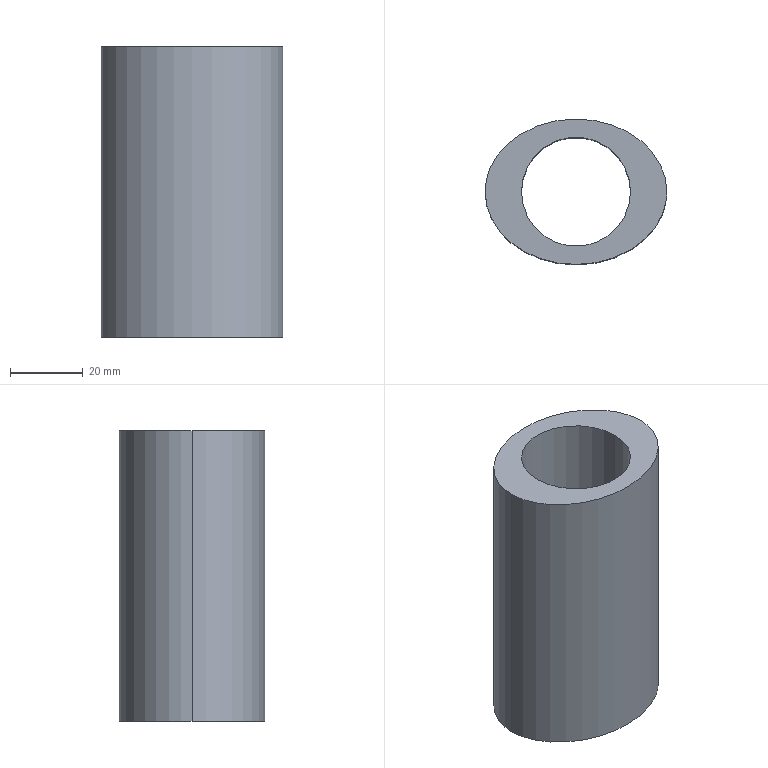Part | SolidWorks | features Extrusion 1, ICE 1 | 1 solid | 6 faces | box 50 x 40 x 80 mm | volume 69122 mm3 | cylinder 2 | spline 2 | plane 2 | commonest cylinder face diameters 30 x2
STEP:
#1=CARTESIAN_POINT('',(-15.,0.,-40.));
#2=VERTEX_POINT('',#1);
#3=CARTESIAN_POINT('',(15.,0.,-40.));
#4=VERTEX_POINT('',#3);
#5=CARTESIAN_POINT('',(0.,0.,-40.));
#6=DIRECTION('',(0.,0.,1.));
#7=DIRECTION('',(1.,0.,0.));
#8=AXIS2_PLACEMENT_3D('',#5,#6,#7);
#9=CIRCLE('',#8,15.);
#10=EDGE_CURVE('',#2,#4,#9,.T.);
#11=ORIENTED_EDGE('',*,*,#10,.F.);
#12=CARTESIAN_POINT('',(-15.,0.,40.));
#13=VERTEX_POINT('',#12);
#14=CARTESIAN_POINT('',(-15.,0.,-40.));
#15=DIRECTION('',(0.,0.,1.));
#16=VECTOR('',#15,1000.);
#17=LINE('',#14,#16);
#18=EDGE_CURVE('',#2,#13,#17,.T.);
#19=ORIENTED_EDGE('',*,*,#18,.T.);
#20=CARTESIAN_POINT('',(15.,0.,40.));
#21=VERTEX_POINT('',#20);
#22=CARTESIAN_POINT('',(0.,0.,40.));
#23=DIRECTION('',(0.,0.,1.));
#24=DIRECTION('',(1.,0.,0.));
#25=AXIS2_PLACEMENT_3D('',#22,#23,#24);
#26=CIRCLE('',#25,15.);
#27=EDGE_CURVE('',#13,#21,#26,.T.);
#28=ORIENTED_EDGE('',*,*,#27,.T.);
#29=CARTESIAN_POINT('',(15.,0.,-40.));
#30=DIRECTION('',(0.,0.,1.));
#31=VECTOR('',#30,1000.);
#32=LINE('',#29,#31);
#33=EDGE_CURVE('',#4,#21,#32,.T.);
#34=ORIENTED_EDGE('',*,*,#33,.F.);
#35=EDGE_LOOP('',(#11,#19,#28,#34));
#36=FACE_OUTER_BOUND('',#35,.T.);
#37=CARTESIAN_POINT('',(0.,0.,-40.));
#38=DIRECTION('',(0.,0.,1.));
#39=DIRECTION('',(1.,0.,0.));
#40=AXIS2_PLACEMENT_3D('',#37,#38,#39);
#41=CYLINDRICAL_SURFACE('',#40,15.);
#42=ADVANCED_FACE('',(#36),#41,.F.);
#43=CARTESIAN_POINT('',(-25.,0.,40.));
#44=VERTEX_POINT('',#43);
#45=CARTESIAN_POINT('',(25.,0.,40.));
#46=VERTEX_POINT('',#45);
#47=CARTESIAN_POINT('',(-25.,0.,40.));
#48=CARTESIAN_POINT('',(-25.,-40.,40.));
#49=CARTESIAN_POINT('',(25.,-40.,40.));
#50=CARTESIAN_POINT('',(25.,0.,40.));
#51=(BOUNDED_CURVE()B_SPLINE_CURVE(3,(#47,#48,#49,#50),.UNSPECIFIED.,.F.,.T.)B_SPLINE_CURVE_WITH_KNOTS((4,4),(3.142,6.283),.UNSPECIFIED.)CURVE()GEOMETRIC_REPRESENTATION_ITEM()RATIONAL_B_SPLINE_CURVE((1.,0.3333,0.3333,1.))REPRESENTATION_ITEM(''));
#52=EDGE_CURVE('',#44,#46,#51,.T.);
#53=ORIENTED_EDGE('',*,*,#52,.F.);
#54=CARTESIAN_POINT('',(-25.,0.,-40.));
#55=VERTEX_POINT('',#54);
#56=CARTESIAN_POINT('',(-25.,0.,40.));
#57=DIRECTION('',(0.,0.,-1.));
#58=VECTOR('',#57,1000.);
#59=LINE('',#56,#58);
#60=EDGE_CURVE('',#44,#55,#59,.T.);
#61=ORIENTED_EDGE('',*,*,#60,.T.);
#62=CARTESIAN_POINT('',(25.,0.,-40.));
#63=VERTEX_POINT('',#62);
#64=CARTESIAN_POINT('',(-25.,0.,-40.));
#65=CARTESIAN_POINT('',(-25.,-40.,-40.));
#66=CARTESIAN_POINT('',(25.,-40.,-40.));
#67=CARTESIAN_POINT('',(25.,0.,-40.));
#68=(BOUNDED_CURVE()B_SPLINE_CURVE(3,(#64,#65,#66,#67),.UNSPECIFIED.,.F.,.T.)B_SPLINE_CURVE_WITH_KNOTS((4,4),(3.142,6.283),.UNSPECIFIED.)CURVE()GEOMETRIC_REPRESENTATION_ITEM()RATIONAL_B_SPLINE_CURVE((1.,0.3333,0.3333,1.))REPRESENTATION_ITEM(''));
#69=EDGE_CURVE('',#55,#63,#68,.T.);
#70=ORIENTED_EDGE('',*,*,#69,.T.);
#71=CARTESIAN_POINT('',(25.,0.,40.));
#72=DIRECTION('',(0.,0.,-1.));
#73=VECTOR('',#72,1000.);
#74=LINE('',#71,#73);
#75=EDGE_CURVE('',#46,#63,#74,.T.);
#76=ORIENTED_EDGE('',*,*,#75,.F.);
#77=EDGE_LOOP('',(#53,#61,#70,#76));
#78=FACE_OUTER_BOUND('',#77,.T.);
#79=CARTESIAN_POINT('',(-25.,0.,40.));
#80=CARTESIAN_POINT('',(-25.,0.,-40.));
#81=CARTESIAN_POINT('',(-25.,-40.,40.));
#82=CARTESIAN_POINT('',(-25.,-40.,-40.));
#83=CARTESIAN_POINT('',(25.,-40.,40.));
#84=CARTESIAN_POINT('',(25.,-40.,-40.));
#85=CARTESIAN_POINT('',(25.,0.,40.));
#86=CARTESIAN_POINT('',(25.,0.,-40.));
#87=(BOUNDED_SURFACE()B_SPLINE_SURFACE(3,1,((#79,#80),(#81,#82),(#83,#84),(#85,#86)),.UNSPECIFIED.,.F.,.F.,.T.)B_SPLINE_SURFACE_WITH_KNOTS((4,4),(2,2),(0.,1.),(0.,1.),.UNSPECIFIED.)GEOMETRIC_REPRESENTATION_ITEM()RATIONAL_B_SPLINE_SURFACE(((1.,1.),(0.3333,0.3333),(0.3333,0.3333),(1.,1.)))REPRESENTATION_ITEM('')SURFACE());
#88=ADVANCED_FACE('',(#78),#87,.F.);
#89=ORIENTED_EDGE('',*,*,#60,.F.);
#90=CARTESIAN_POINT('',(25.,0.,40.));
#91=CARTESIAN_POINT('',(25.,40.,40.));
#92=CARTESIAN_POINT('',(-25.,40.,40.));
#93=CARTESIAN_POINT('',(-25.,0.,40.));
#94=(BOUNDED_CURVE()B_SPLINE_CURVE(3,(#90,#91,#92,#93),.UNSPECIFIED.,.F.,.T.)B_SPLINE_CURVE_WITH_KNOTS((4,4),(0.,3.142),.UNSPECIFIED.)CURVE()GEOMETRIC_REPRESENTATION_ITEM()RATIONAL_B_SPLINE_CURVE((1.,0.3333,0.3333,1.))REPRESENTATION_ITEM(''));
#95=EDGE_CURVE('',#46,#44,#94,.T.);
#96=ORIENTED_EDGE('',*,*,#95,.F.);
#97=ORIENTED_EDGE('',*,*,#75,.T.);
#98=CARTESIAN_POINT('',(25.,0.,-40.));
#99=CARTESIAN_POINT('',(25.,40.,-40.));
#100=CARTESIAN_POINT('',(-25.,40.,-40.));
#101=CARTESIAN_POINT('',(-25.,0.,-40.));
#102=(BOUNDED_CURVE()B_SPLINE_CURVE(3,(#98,#99,#100,#101),.UNSPECIFIED.,.F.,.T.)B_SPLINE_CURVE_WITH_KNOTS((4,4),(0.,3.142),.UNSPECIFIED.)CURVE()GEOMETRIC_REPRESENTATION_ITEM()RATIONAL_B_SPLINE_CURVE((1.,0.3333,0.3333,1.))REPRESENTATION_ITEM(''));
#103=EDGE_CURVE('',#63,#55,#102,.T.);
#104=ORIENTED_EDGE('',*,*,#103,.T.);
#105=EDGE_LOOP('',(#89,#96,#97,#104));
#106=FACE_OUTER_BOUND('',#105,.T.);
#107=CARTESIAN_POINT('',(25.,0.,40.));
#108=CARTESIAN_POINT('',(25.,0.,-40.));
#109=CARTESIAN_POINT('',(25.,40.,40.));
#110=CARTESIAN_POINT('',(25.,40.,-40.));
#111=CARTESIAN_POINT('',(-25.,40.,40.));
#112=CARTESIAN_POINT('',(-25.,40.,-40.));
#113=CARTESIAN_POINT('',(-25.,0.,40.));
#114=CARTESIAN_POINT('',(-25.,0.,-40.));
#115=(BOUNDED_SURFACE()B_SPLINE_SURFACE(3,1,((#107,#108),(#109,#110),(#111,#112),(#113,#114)),.UNSPECIFIED.,.F.,.F.,.T.)B_SPLINE_SURFACE_WITH_KNOTS((4,4),(2,2),(0.,1.),(0.,1.),.UNSPECIFIED.)GEOMETRIC_REPRESENTATION_ITEM()RATIONAL_B_SPLINE_SURFACE(((1.,1.),(0.3333,0.3333),(0.3333,0.3333),(1.,1.)))REPRESENTATION_ITEM('')SURFACE());
#116=ADVANCED_FACE('',(#106),#115,.F.);
#117=CARTESIAN_POINT('',(0.,0.,40.));
#118=DIRECTION('',(0.,0.,1.));
#119=DIRECTION('',(1.,0.,0.));
#120=AXIS2_PLACEMENT_3D('',#117,#118,#119);
#121=CIRCLE('',#120,15.);
#122=EDGE_CURVE('',#21,#13,#121,.T.);
#123=ORIENTED_EDGE('',*,*,#122,.F.);
#124=ORIENTED_EDGE('',*,*,#27,.F.);
#125=EDGE_LOOP('',(#123,#124));
#126=FACE_BOUND('',#125,.T.);
#127=ORIENTED_EDGE('',*,*,#95,.T.);
#128=ORIENTED_EDGE('',*,*,#52,.T.);
#129=EDGE_LOOP('',(#127,#128));
#130=FACE_OUTER_BOUND('',#129,.T.);
#131=CARTESIAN_POINT('',(0.,0.,40.));
#132=DIRECTION('',(0.,0.,1.));
#133=DIRECTION('',(1.,0.,0.));
#134=AXIS2_PLACEMENT_3D('',#131,#132,#133);
#135=PLANE('',#134);
#136=ADVANCED_FACE('',(#126,#130),#135,.T.);
#137=CARTESIAN_POINT('',(0.,0.,-40.));
#138=DIRECTION('',(0.,0.,1.));
#139=DIRECTION('',(1.,0.,0.));
#140=AXIS2_PLACEMENT_3D('',#137,#138,#139);
#141=CIRCLE('',#140,15.);
#142=EDGE_CURVE('',#4,#2,#141,.T.);
#143=ORIENTED_EDGE('',*,*,#142,.T.);
#144=ORIENTED_EDGE('',*,*,#10,.T.);
#145=EDGE_LOOP('',(#143,#144));
#146=FACE_BOUND('',#145,.T.);
#147=ORIENTED_EDGE('',*,*,#103,.F.);
#148=ORIENTED_EDGE('',*,*,#69,.F.);
#149=EDGE_LOOP('',(#147,#148));
#150=FACE_OUTER_BOUND('',#149,.T.);
#151=CARTESIAN_POINT('',(0.,0.,-40.));
#152=DIRECTION('',(0.,0.,1.));
#153=DIRECTION('',(1.,0.,0.));
#154=AXIS2_PLACEMENT_3D('',#151,#152,#153);
#155=PLANE('',#154);
#156=ADVANCED_FACE('',(#146,#150),#155,.F.);
#157=ORIENTED_EDGE('',*,*,#18,.F.);
#158=ORIENTED_EDGE('',*,*,#142,.F.);
#159=ORIENTED_EDGE('',*,*,#33,.T.);
#160=ORIENTED_EDGE('',*,*,#122,.T.);
#161=EDGE_LOOP('',(#157,#158,#159,#160));
#162=FACE_OUTER_BOUND('',#161,.T.);
#163=CARTESIAN_POINT('',(0.,0.,-40.));
#164=DIRECTION('',(0.,0.,1.));
#165=DIRECTION('',(1.,0.,0.));
#166=AXIS2_PLACEMENT_3D('',#163,#164,#165);
#167=CYLINDRICAL_SURFACE('',#166,15.);
#168=ADVANCED_FACE('',(#162),#167,.F.);
#169=CLOSED_SHELL('',(#42,#88,#116,#136,#156,#168));
#170=MANIFOLD_SOLID_BREP('',#169);
#171=CARTESIAN_POINT('',(0.,0.,0.));
#172=DIRECTION('',(0.,0.,1.));
#173=DIRECTION('',(1.,0.,0.));
#174=AXIS2_PLACEMENT_3D('',#171,#172,#173);
#175=(LENGTH_UNIT()NAMED_UNIT(*)SI_UNIT(.MILLI.,.METRE.));
#176=UNCERTAINTY_MEASURE_WITH_UNIT(LENGTH_MEASURE(0.00001),#175,'','');
#177=(NAMED_UNIT(*)PLANE_ANGLE_UNIT()SI_UNIT($,.RADIAN.));
#178=(NAMED_UNIT(*)SI_UNIT($,.STERADIAN.)SOLID_ANGLE_UNIT());
#179=(GEOMETRIC_REPRESENTATION_CONTEXT(3)GLOBAL_UNCERTAINTY_ASSIGNED_CONTEXT((#176))GLOBAL_UNIT_ASSIGNED_CONTEXT((#175,#177,#178))REPRESENTATION_CONTEXT('',''));
#180=ADVANCED_BREP_SHAPE_REPRESENTATION('',(#170,#174),#179);